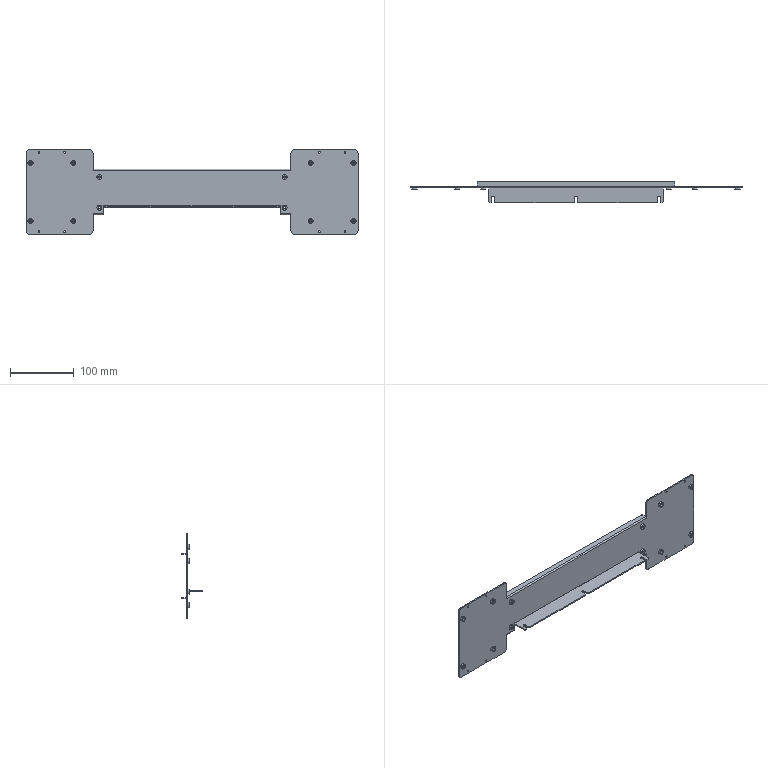Part | STEP file | 9 solids | 188 faces | box 520 x 33 x 132 mm | volume 111662 mm3 | cylinder 105 | plane 83 | commonest cylinder face diameters 3.3 x24 8 x24 2.5 x16 4.5 x16 10 x8 4.2 x7